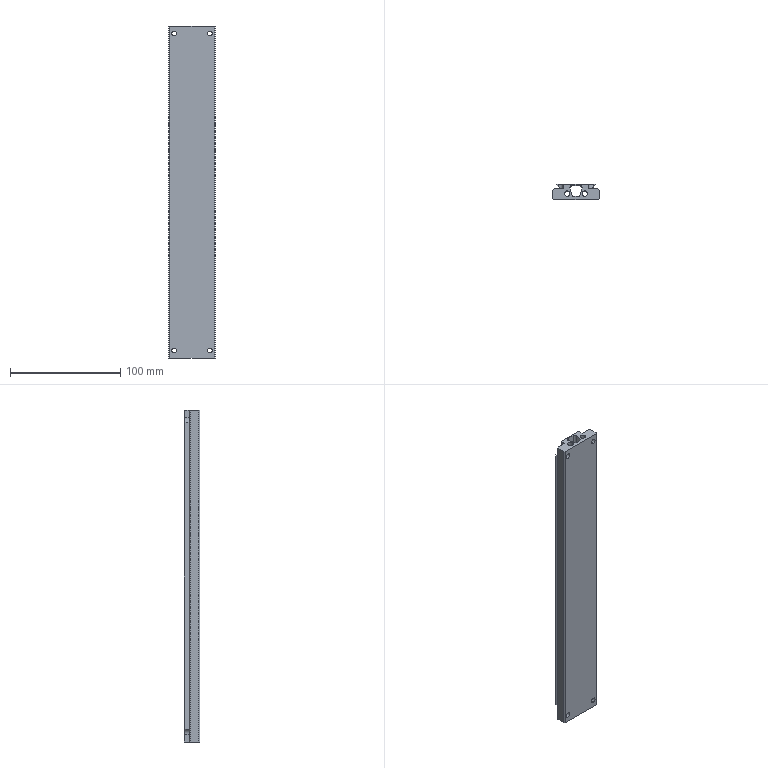Part | STEP file | P193372_BVP_HMPL_12_100 | 1 solid | 59 faces | box 42 x 14 x 301.6 mm | volume 121442 mm3 | plane 30 | cylinder 29 | commonest cylinder face diameters 4.5 x8 8 x8 5 x4 10 x4 0.5 x3 4.8 x2